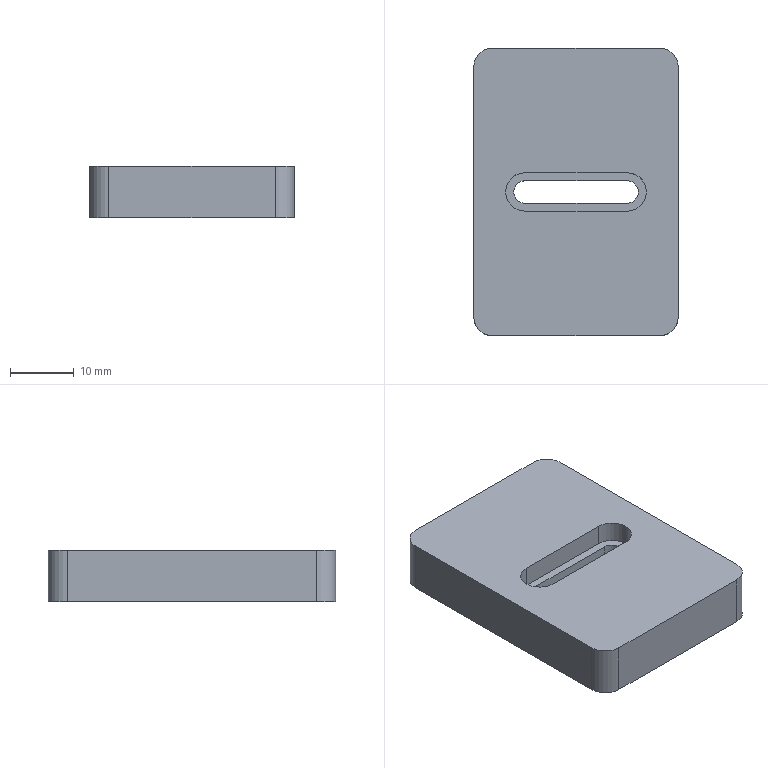Part | SolidWorks | features HoleWzd 2, ICE 2, Extrusion 1, Fillet 1 | 1 solid | 21 faces | box 32 x 45 x 8 mm | volume 10740 mm3 | plane 11 | cylinder 10 | commonest cylinder face diameters 6 x7 3.5 x3
STEP:
#1=CARTESIAN_POINT('',(11.,0.,4.7));
#2=VERTEX_POINT('',#1);
#3=CARTESIAN_POINT('',(8.,3.,4.7));
#4=VERTEX_POINT('',#3);
#5=CARTESIAN_POINT('',(8.,0.,4.7));
#6=DIRECTION('',(0.,0.,1.));
#7=DIRECTION('',(1.,0.,0.));
#8=AXIS2_PLACEMENT_3D('',#5,#6,#7);
#9=CIRCLE('',#8,3.);
#10=EDGE_CURVE('',#2,#4,#9,.T.);
#11=ORIENTED_EDGE('',*,*,#10,.F.);
#12=CARTESIAN_POINT('',(11.,0.,8.));
#13=VERTEX_POINT('',#12);
#14=CARTESIAN_POINT('',(11.,0.,4.7));
#15=DIRECTION('',(0.,0.,1.));
#16=VECTOR('',#15,1000.);
#17=LINE('',#14,#16);
#18=EDGE_CURVE('',#2,#13,#17,.T.);
#19=ORIENTED_EDGE('',*,*,#18,.T.);
#20=CARTESIAN_POINT('',(8.,3.,8.));
#21=VERTEX_POINT('',#20);
#22=CARTESIAN_POINT('',(8.,0.,8.));
#23=DIRECTION('',(0.,0.,1.));
#24=DIRECTION('',(1.,0.,0.));
#25=AXIS2_PLACEMENT_3D('',#22,#23,#24);
#26=CIRCLE('',#25,3.);
#27=EDGE_CURVE('',#13,#21,#26,.T.);
#28=ORIENTED_EDGE('',*,*,#27,.T.);
#29=CARTESIAN_POINT('',(8.,3.,4.7));
#30=DIRECTION('',(0.,0.,1.));
#31=VECTOR('',#30,1000.);
#32=LINE('',#29,#31);
#33=EDGE_CURVE('',#4,#21,#32,.T.);
#34=ORIENTED_EDGE('',*,*,#33,.F.);
#35=EDGE_LOOP('',(#11,#19,#28,#34));
#36=FACE_OUTER_BOUND('',#35,.T.);
#37=CARTESIAN_POINT('',(8.,0.,4.7));
#38=DIRECTION('',(0.,0.,1.));
#39=DIRECTION('',(1.,0.,0.));
#40=AXIS2_PLACEMENT_3D('',#37,#38,#39);
#41=CYLINDRICAL_SURFACE('',#40,3.);
#42=ADVANCED_FACE('',(#36),#41,.F.);
#43=CARTESIAN_POINT('',(9.75,0.,0.));
#44=VERTEX_POINT('',#43);
#45=CARTESIAN_POINT('',(8.,1.75,0.));
#46=VERTEX_POINT('',#45);
#47=CARTESIAN_POINT('',(8.,0.,0.));
#48=DIRECTION('',(0.,0.,1.));
#49=DIRECTION('',(1.,0.,0.));
#50=AXIS2_PLACEMENT_3D('',#47,#48,#49);
#51=CIRCLE('',#50,1.75);
#52=EDGE_CURVE('',#44,#46,#51,.T.);
#53=ORIENTED_EDGE('',*,*,#52,.F.);
#54=CARTESIAN_POINT('',(9.75,0.,4.7));
#55=VERTEX_POINT('',#54);
#56=CARTESIAN_POINT('',(9.75,0.,0.));
#57=DIRECTION('',(0.,0.,1.));
#58=VECTOR('',#57,1000.);
#59=LINE('',#56,#58);
#60=EDGE_CURVE('',#44,#55,#59,.T.);
#61=ORIENTED_EDGE('',*,*,#60,.T.);
#62=CARTESIAN_POINT('',(8.,1.75,4.7));
#63=VERTEX_POINT('',#62);
#64=CARTESIAN_POINT('',(8.,0.,4.7));
#65=DIRECTION('',(0.,0.,-1.));
#66=DIRECTION('',(1.,0.,0.));
#67=AXIS2_PLACEMENT_3D('',#64,#65,#66);
#68=CIRCLE('',#67,1.75);
#69=EDGE_CURVE('',#63,#55,#68,.T.);
#70=ORIENTED_EDGE('',*,*,#69,.F.);
#71=CARTESIAN_POINT('',(8.,1.75,0.));
#72=DIRECTION('',(0.,0.,1.));
#73=VECTOR('',#72,1000.);
#74=LINE('',#71,#73);
#75=EDGE_CURVE('',#46,#63,#74,.T.);
#76=ORIENTED_EDGE('',*,*,#75,.F.);
#77=EDGE_LOOP('',(#53,#61,#70,#76));
#78=FACE_OUTER_BOUND('',#77,.T.);
#79=CARTESIAN_POINT('',(8.,0.,0.));
#80=DIRECTION('',(0.,0.,1.));
#81=DIRECTION('',(1.,0.,0.));
#82=AXIS2_PLACEMENT_3D('',#79,#80,#81);
#83=CYLINDRICAL_SURFACE('',#82,1.75);
#84=ADVANCED_FACE('',(#78),#83,.F.);
#85=CARTESIAN_POINT('',(-8.,-1.75,4.7));
#86=VERTEX_POINT('',#85);
#87=CARTESIAN_POINT('',(-8.,1.75,4.7));
#88=VERTEX_POINT('',#87);
#89=CARTESIAN_POINT('',(-8.,0.,4.7));
#90=DIRECTION('',(0.,0.,-1.));
#91=DIRECTION('',(1.,0.,0.));
#92=AXIS2_PLACEMENT_3D('',#89,#90,#91);
#93=CIRCLE('',#92,1.75);
#94=EDGE_CURVE('',#86,#88,#93,.T.);
#95=ORIENTED_EDGE('',*,*,#94,.F.);
#96=CARTESIAN_POINT('',(-8.,-1.75,0.));
#97=VERTEX_POINT('',#96);
#98=CARTESIAN_POINT('',(-8.,-1.75,0.));
#99=DIRECTION('',(0.,0.,1.));
#100=VECTOR('',#99,1000.);
#101=LINE('',#98,#100);
#102=EDGE_CURVE('',#97,#86,#101,.T.);
#103=ORIENTED_EDGE('',*,*,#102,.F.);
#104=CARTESIAN_POINT('',(-8.,1.75,0.));
#105=VERTEX_POINT('',#104);
#106=CARTESIAN_POINT('',(-8.,0.,0.));
#107=DIRECTION('',(0.,0.,1.));
#108=DIRECTION('',(1.,0.,0.));
#109=AXIS2_PLACEMENT_3D('',#106,#107,#108);
#110=CIRCLE('',#109,1.75);
#111=EDGE_CURVE('',#105,#97,#110,.T.);
#112=ORIENTED_EDGE('',*,*,#111,.F.);
#113=CARTESIAN_POINT('',(-8.,1.75,0.));
#114=DIRECTION('',(0.,0.,1.));
#115=VECTOR('',#114,1000.);
#116=LINE('',#113,#115);
#117=EDGE_CURVE('',#105,#88,#116,.T.);
#118=ORIENTED_EDGE('',*,*,#117,.T.);
#119=EDGE_LOOP('',(#95,#103,#112,#118));
#120=FACE_OUTER_BOUND('',#119,.T.);
#121=CARTESIAN_POINT('',(-8.,0.,0.));
#122=DIRECTION('',(0.,0.,1.));
#123=DIRECTION('',(1.,0.,0.));
#124=AXIS2_PLACEMENT_3D('',#121,#122,#123);
#125=CYLINDRICAL_SURFACE('',#124,1.75);
#126=ADVANCED_FACE('',(#120),#125,.F.);
#127=CARTESIAN_POINT('',(-8.,1.75,4.7));
#128=DIRECTION('',(1.,0.,0.));
#129=VECTOR('',#128,1000.);
#130=LINE('',#127,#129);
#131=EDGE_CURVE('',#88,#63,#130,.T.);
#132=ORIENTED_EDGE('',*,*,#131,.F.);
#133=ORIENTED_EDGE('',*,*,#117,.F.);
#134=CARTESIAN_POINT('',(-8.,1.75,0.));
#135=DIRECTION('',(-1.,0.,0.));
#136=VECTOR('',#135,1000.);
#137=LINE('',#134,#136);
#138=EDGE_CURVE('',#46,#105,#137,.T.);
#139=ORIENTED_EDGE('',*,*,#138,.F.);
#140=ORIENTED_EDGE('',*,*,#75,.T.);
#141=EDGE_LOOP('',(#132,#133,#139,#140));
#142=FACE_OUTER_BOUND('',#141,.T.);
#143=CARTESIAN_POINT('',(-8.,1.75,0.));
#144=DIRECTION('',(0.,1.,0.));
#145=DIRECTION('',(0.,0.,1.));
#146=AXIS2_PLACEMENT_3D('',#143,#144,#145);
#147=PLANE('',#146);
#148=ADVANCED_FACE('',(#142),#147,.F.);
#149=ORIENTED_EDGE('',*,*,#60,.F.);
#150=CARTESIAN_POINT('',(8.,-1.75,0.));
#151=VERTEX_POINT('',#150);
#152=CARTESIAN_POINT('',(8.,0.,0.));
#153=DIRECTION('',(0.,0.,1.));
#154=DIRECTION('',(1.,0.,0.));
#155=AXIS2_PLACEMENT_3D('',#152,#153,#154);
#156=CIRCLE('',#155,1.75);
#157=EDGE_CURVE('',#151,#44,#156,.T.);
#158=ORIENTED_EDGE('',*,*,#157,.F.);
#159=CARTESIAN_POINT('',(8.,-1.75,4.7));
#160=VERTEX_POINT('',#159);
#161=CARTESIAN_POINT('',(8.,-1.75,0.));
#162=DIRECTION('',(0.,0.,1.));
#163=VECTOR('',#162,1000.);
#164=LINE('',#161,#163);
#165=EDGE_CURVE('',#151,#160,#164,.T.);
#166=ORIENTED_EDGE('',*,*,#165,.T.);
#167=CARTESIAN_POINT('',(8.,0.,4.7));
#168=DIRECTION('',(0.,0.,-1.));
#169=DIRECTION('',(1.,0.,0.));
#170=AXIS2_PLACEMENT_3D('',#167,#168,#169);
#171=CIRCLE('',#170,1.75);
#172=EDGE_CURVE('',#55,#160,#171,.T.);
#173=ORIENTED_EDGE('',*,*,#172,.F.);
#174=EDGE_LOOP('',(#149,#158,#166,#173));
#175=FACE_OUTER_BOUND('',#174,.T.);
#176=CARTESIAN_POINT('',(8.,0.,0.));
#177=DIRECTION('',(0.,0.,1.));
#178=DIRECTION('',(1.,0.,0.));
#179=AXIS2_PLACEMENT_3D('',#176,#177,#178);
#180=CYLINDRICAL_SURFACE('',#179,1.75);
#181=ADVANCED_FACE('',(#175),#180,.F.);
#182=CARTESIAN_POINT('',(-8.,-1.75,4.7));
#183=DIRECTION('',(-1.,0.,0.));
#184=VECTOR('',#183,1000.);
#185=LINE('',#182,#184);
#186=EDGE_CURVE('',#160,#86,#185,.T.);
#187=ORIENTED_EDGE('',*,*,#186,.F.);
#188=ORIENTED_EDGE('',*,*,#165,.F.);
#189=CARTESIAN_POINT('',(-8.,-1.75,0.));
#190=DIRECTION('',(1.,0.,0.));
#191=VECTOR('',#190,1000.);
#192=LINE('',#189,#191);
#193=EDGE_CURVE('',#97,#151,#192,.T.);
#194=ORIENTED_EDGE('',*,*,#193,.F.);
#195=ORIENTED_EDGE('',*,*,#102,.T.);
#196=EDGE_LOOP('',(#187,#188,#194,#195));
#197=FACE_OUTER_BOUND('',#196,.T.);
#198=CARTESIAN_POINT('',(-8.,-1.75,0.));
#199=DIRECTION('',(0.,-1.,0.));
#200=DIRECTION('',(0.,0.,-1.));
#201=AXIS2_PLACEMENT_3D('',#198,#199,#200);
#202=PLANE('',#201);
#203=ADVANCED_FACE('',(#197),#202,.F.);
#204=CARTESIAN_POINT('',(-16.,19.5,8.));
#205=VERTEX_POINT('',#204);
#206=CARTESIAN_POINT('',(-16.,-19.5,8.));
#207=VERTEX_POINT('',#206);
#208=CARTESIAN_POINT('',(-16.,-22.5,8.));
#209=DIRECTION('',(0.,-1.,0.));
#210=VECTOR('',#209,1000.);
#211=LINE('',#208,#210);
#212=EDGE_CURVE('',#205,#207,#211,.T.);
#213=ORIENTED_EDGE('',*,*,#212,.F.);
#214=CARTESIAN_POINT('',(-16.,19.5,0.));
#215=VERTEX_POINT('',#214);
#216=CARTESIAN_POINT('',(-16.,19.5,8.));
#217=DIRECTION('',(0.,0.,-1.));
#218=VECTOR('',#217,1000.);
#219=LINE('',#216,#218);
#220=EDGE_CURVE('',#205,#215,#219,.T.);
#221=ORIENTED_EDGE('',*,*,#220,.T.);
#222=CARTESIAN_POINT('',(-16.,-19.5,0.));
#223=VERTEX_POINT('',#222);
#224=CARTESIAN_POINT('',(-16.,-22.5,0.));
#225=DIRECTION('',(0.,-1.,0.));
#226=VECTOR('',#225,1000.);
#227=LINE('',#224,#226);
#228=EDGE_CURVE('',#215,#223,#227,.T.);
#229=ORIENTED_EDGE('',*,*,#228,.T.);
#230=CARTESIAN_POINT('',(-16.,-19.5,8.));
#231=DIRECTION('',(0.,0.,1.));
#232=VECTOR('',#231,1000.);
#233=LINE('',#230,#232);
#234=EDGE_CURVE('',#223,#207,#233,.T.);
#235=ORIENTED_EDGE('',*,*,#234,.T.);
#236=EDGE_LOOP('',(#213,#221,#229,#235));
#237=FACE_OUTER_BOUND('',#236,.T.);
#238=CARTESIAN_POINT('',(-16.,-22.5,8.));
#239=DIRECTION('',(1.,0.,0.));
#240=DIRECTION('',(0.,0.,-1.));
#241=AXIS2_PLACEMENT_3D('',#238,#239,#240);
#242=PLANE('',#241);
#243=ADVANCED_FACE('',(#237),#242,.F.);
#244=CARTESIAN_POINT('',(-13.,-22.5,0.));
#245=VERTEX_POINT('',#244);
#246=CARTESIAN_POINT('',(13.,-22.5,0.));
#247=VERTEX_POINT('',#246);
#248=CARTESIAN_POINT('',(16.,-22.5,0.));
#249=DIRECTION('',(1.,0.,0.));
#250=VECTOR('',#249,1000.);
#251=LINE('',#248,#250);
#252=EDGE_CURVE('',#245,#247,#251,.T.);
#253=ORIENTED_EDGE('',*,*,#252,.T.);
#254=CARTESIAN_POINT('',(13.,-22.5,8.));
#255=VERTEX_POINT('',#254);
#256=CARTESIAN_POINT('',(13.,-22.5,8.));
#257=DIRECTION('',(0.,0.,1.));
#258=VECTOR('',#257,1000.);
#259=LINE('',#256,#258);
#260=EDGE_CURVE('',#247,#255,#259,.T.);
#261=ORIENTED_EDGE('',*,*,#260,.T.);
#262=CARTESIAN_POINT('',(-13.,-22.5,8.));
#263=VERTEX_POINT('',#262);
#264=CARTESIAN_POINT('',(16.,-22.5,8.));
#265=DIRECTION('',(1.,0.,0.));
#266=VECTOR('',#265,1000.);
#267=LINE('',#264,#266);
#268=EDGE_CURVE('',#263,#255,#267,.T.);
#269=ORIENTED_EDGE('',*,*,#268,.F.);
#270=CARTESIAN_POINT('',(-13.,-22.5,8.));
#271=DIRECTION('',(0.,0.,-1.));
#272=VECTOR('',#271,1000.);
#273=LINE('',#270,#272);
#274=EDGE_CURVE('',#263,#245,#273,.T.);
#275=ORIENTED_EDGE('',*,*,#274,.T.);
#276=EDGE_LOOP('',(#253,#261,#269,#275));
#277=FACE_OUTER_BOUND('',#276,.T.);
#278=CARTESIAN_POINT('',(16.,-22.5,8.));
#279=DIRECTION('',(0.,1.,0.));
#280=DIRECTION('',(-1.,0.,0.));
#281=AXIS2_PLACEMENT_3D('',#278,#279,#280);
#282=PLANE('',#281);
#283=ADVANCED_FACE('',(#277),#282,.F.);
#284=CARTESIAN_POINT('',(16.,-19.5,0.));
#285=VERTEX_POINT('',#284);
#286=CARTESIAN_POINT('',(16.,19.5,0.));
#287=VERTEX_POINT('',#286);
#288=CARTESIAN_POINT('',(16.,-22.5,0.));
#289=DIRECTION('',(0.,1.,0.));
#290=VECTOR('',#289,1000.);
#291=LINE('',#288,#290);
#292=EDGE_CURVE('',#285,#287,#291,.T.);
#293=ORIENTED_EDGE('',*,*,#292,.T.);
#294=CARTESIAN_POINT('',(16.,19.5,8.));
#295=VERTEX_POINT('',#294);
#296=CARTESIAN_POINT('',(16.,19.5,8.));
#297=DIRECTION('',(0.,0.,1.));
#298=VECTOR('',#297,1000.);
#299=LINE('',#296,#298);
#300=EDGE_CURVE('',#287,#295,#299,.T.);
#301=ORIENTED_EDGE('',*,*,#300,.T.);
#302=CARTESIAN_POINT('',(16.,-19.5,8.));
#303=VERTEX_POINT('',#302);
#304=CARTESIAN_POINT('',(16.,-22.5,8.));
#305=DIRECTION('',(0.,1.,0.));
#306=VECTOR('',#305,1000.);
#307=LINE('',#304,#306);
#308=EDGE_CURVE('',#303,#295,#307,.T.);
#309=ORIENTED_EDGE('',*,*,#308,.F.);
#310=CARTESIAN_POINT('',(16.,-19.5,8.));
#311=DIRECTION('',(0.,0.,-1.));
#312=VECTOR('',#311,1000.);
#313=LINE('',#310,#312);
#314=EDGE_CURVE('',#303,#285,#313,.T.);
#315=ORIENTED_EDGE('',*,*,#314,.T.);
#316=EDGE_LOOP('',(#293,#301,#309,#315));
#317=FACE_OUTER_BOUND('',#316,.T.);
#318=CARTESIAN_POINT('',(16.,-22.5,8.));
#319=DIRECTION('',(-1.,0.,0.));
#320=DIRECTION('',(0.,0.,1.));
#321=AXIS2_PLACEMENT_3D('',#318,#319,#320);
#322=PLANE('',#321);
#323=ADVANCED_FACE('',(#317),#322,.F.);
#324=CARTESIAN_POINT('',(13.,22.5,0.));
#325=VERTEX_POINT('',#324);
#326=CARTESIAN_POINT('',(-13.,22.5,0.));
#327=VERTEX_POINT('',#326);
#328=CARTESIAN_POINT('',(16.,22.5,0.));
#329=DIRECTION('',(-1.,0.,0.));
#330=VECTOR('',#329,1000.);
#331=LINE('',#328,#330);
#332=EDGE_CURVE('',#325,#327,#331,.T.);
#333=ORIENTED_EDGE('',*,*,#332,.T.);
#334=CARTESIAN_POINT('',(-13.,22.5,8.));
#335=VERTEX_POINT('',#334);
#336=CARTESIAN_POINT('',(-13.,22.5,8.));
#337=DIRECTION('',(0.,0.,1.));
#338=VECTOR('',#337,1000.);
#339=LINE('',#336,#338);
#340=EDGE_CURVE('',#327,#335,#339,.T.);
#341=ORIENTED_EDGE('',*,*,#340,.T.);
#342=CARTESIAN_POINT('',(13.,22.5,8.));
#343=VERTEX_POINT('',#342);
#344=CARTESIAN_POINT('',(16.,22.5,8.));
#345=DIRECTION('',(-1.,0.,0.));
#346=VECTOR('',#345,1000.);
#347=LINE('',#344,#346);
#348=EDGE_CURVE('',#343,#335,#347,.T.);
#349=ORIENTED_EDGE('',*,*,#348,.F.);
#350=CARTESIAN_POINT('',(13.,22.5,8.));
#351=DIRECTION('',(0.,0.,-1.));
#352=VECTOR('',#351,1000.);
#353=LINE('',#350,#352);
#354=EDGE_CURVE('',#343,#325,#353,.T.);
#355=ORIENTED_EDGE('',*,*,#354,.T.);
#356=EDGE_LOOP('',(#333,#341,#349,#355));
#357=FACE_OUTER_BOUND('',#356,.T.);
#358=CARTESIAN_POINT('',(16.,22.5,8.));
#359=DIRECTION('',(0.,-1.,0.));
#360=DIRECTION('',(1.,0.,0.));
#361=AXIS2_PLACEMENT_3D('',#358,#359,#360);
#362=PLANE('',#361);
#363=ADVANCED_FACE('',(#357),#362,.F.);
#364=CARTESIAN_POINT('',(-8.,3.,8.));
#365=VERTEX_POINT('',#364);
#366=CARTESIAN_POINT('',(-8.,-3.,8.));
#367=VERTEX_POINT('',#366);
#368=CARTESIAN_POINT('',(-8.,0.,8.));
#369=DIRECTION('',(0.,0.,1.));
#370=DIRECTION('',(1.,0.,0.));
#371=AXIS2_PLACEMENT_3D('',#368,#369,#370);
#372=CIRCLE('',#371,3.);
#373=EDGE_CURVE('',#365,#367,#372,.T.);
#374=ORIENTED_EDGE('',*,*,#373,.F.);
#375=CARTESIAN_POINT('',(-8.,3.,8.));
#376=DIRECTION('',(-1.,0.,0.));
#377=VECTOR('',#376,1000.);
#378=LINE('',#375,#377);
#379=EDGE_CURVE('',#21,#365,#378,.T.);
#380=ORIENTED_EDGE('',*,*,#379,.F.);
#381=ORIENTED_EDGE('',*,*,#27,.F.);
#382=CARTESIAN_POINT('',(8.,-3.,8.));
#383=VERTEX_POINT('',#382);
#384=CARTESIAN_POINT('',(8.,0.,8.));
#385=DIRECTION('',(0.,0.,1.));
#386=DIRECTION('',(1.,0.,0.));
#387=AXIS2_PLACEMENT_3D('',#384,#385,#386);
#388=CIRCLE('',#387,3.);
#389=EDGE_CURVE('',#383,#13,#388,.T.);
#390=ORIENTED_EDGE('',*,*,#389,.F.);
#391=CARTESIAN_POINT('',(-8.,-3.,8.));
#392=DIRECTION('',(1.,0.,0.));
#393=VECTOR('',#392,1000.);
#394=LINE('',#391,#393);
#395=EDGE_CURVE('',#367,#383,#394,.T.);
#396=ORIENTED_EDGE('',*,*,#395,.F.);
#397=EDGE_LOOP('',(#374,#380,#381,#390,#396));
#398=FACE_BOUND('',#397,.T.);
#399=ORIENTED_EDGE('',*,*,#348,.T.);
#400=CARTESIAN_POINT('',(-13.,19.5,8.));
#401=DIRECTION('',(0.,0.,1.));
#402=DIRECTION('',(1.,0.,0.));
#403=AXIS2_PLACEMENT_3D('',#400,#401,#402);
#404=CIRCLE('',#403,3.);
#405=EDGE_CURVE('',#335,#205,#404,.T.);
#406=ORIENTED_EDGE('',*,*,#405,.T.);
#407=ORIENTED_EDGE('',*,*,#212,.T.);
#408=CARTESIAN_POINT('',(-13.,-19.5,8.));
#409=DIRECTION('',(0.,0.,1.));
#410=DIRECTION('',(1.,0.,0.));
#411=AXIS2_PLACEMENT_3D('',#408,#409,#410);
#412=CIRCLE('',#411,3.);
#413=EDGE_CURVE('',#207,#263,#412,.T.);
#414=ORIENTED_EDGE('',*,*,#413,.T.);
#415=ORIENTED_EDGE('',*,*,#268,.T.);
#416=CARTESIAN_POINT('',(13.,-19.5,8.));
#417=DIRECTION('',(0.,0.,1.));
#418=DIRECTION('',(1.,0.,0.));
#419=AXIS2_PLACEMENT_3D('',#416,#417,#418);
#420=CIRCLE('',#419,3.);
#421=EDGE_CURVE('',#255,#303,#420,.T.);
#422=ORIENTED_EDGE('',*,*,#421,.T.);
#423=ORIENTED_EDGE('',*,*,#308,.T.);
#424=CARTESIAN_POINT('',(13.,19.5,8.));
#425=DIRECTION('',(0.,0.,1.));
#426=DIRECTION('',(1.,0.,0.));
#427=AXIS2_PLACEMENT_3D('',#424,#425,#426);
#428=CIRCLE('',#427,3.);
#429=EDGE_CURVE('',#295,#343,#428,.T.);
#430=ORIENTED_EDGE('',*,*,#429,.T.);
#431=EDGE_LOOP('',(#399,#406,#407,#414,#415,#422,#423,#430));
#432=FACE_OUTER_BOUND('',#431,.T.);
#433=CARTESIAN_POINT('',(0.,0.,8.));
#434=DIRECTION('',(0.,0.,1.));
#435=DIRECTION('',(1.,0.,0.));
#436=AXIS2_PLACEMENT_3D('',#433,#434,#435);
#437=PLANE('',#436);
#438=ADVANCED_FACE('',(#398,#432),#437,.T.);
#439=ORIENTED_EDGE('',*,*,#138,.T.);
#440=ORIENTED_EDGE('',*,*,#111,.T.);
#441=ORIENTED_EDGE('',*,*,#193,.T.);
#442=ORIENTED_EDGE('',*,*,#157,.T.);
#443=ORIENTED_EDGE('',*,*,#52,.T.);
#444=EDGE_LOOP('',(#439,#440,#441,#442,#443));
#445=FACE_BOUND('',#444,.T.);
#446=ORIENTED_EDGE('',*,*,#228,.F.);
#447=CARTESIAN_POINT('',(-13.,19.5,0.));
#448=DIRECTION('',(0.,0.,-1.));
#449=DIRECTION('',(1.,0.,0.));
#450=AXIS2_PLACEMENT_3D('',#447,#448,#449);
#451=CIRCLE('',#450,3.);
#452=EDGE_CURVE('',#215,#327,#451,.T.);
#453=ORIENTED_EDGE('',*,*,#452,.T.);
#454=ORIENTED_EDGE('',*,*,#332,.F.);
#455=CARTESIAN_POINT('',(13.,19.5,0.));
#456=DIRECTION('',(0.,0.,-1.));
#457=DIRECTION('',(1.,0.,0.));
#458=AXIS2_PLACEMENT_3D('',#455,#456,#457);
#459=CIRCLE('',#458,3.);
#460=EDGE_CURVE('',#325,#287,#459,.T.);
#461=ORIENTED_EDGE('',*,*,#460,.T.);
#462=ORIENTED_EDGE('',*,*,#292,.F.);
#463=CARTESIAN_POINT('',(13.,-19.5,0.));
#464=DIRECTION('',(0.,0.,-1.));
#465=DIRECTION('',(1.,0.,0.));
#466=AXIS2_PLACEMENT_3D('',#463,#464,#465);
#467=CIRCLE('',#466,3.);
#468=EDGE_CURVE('',#285,#247,#467,.T.);
#469=ORIENTED_EDGE('',*,*,#468,.T.);
#470=ORIENTED_EDGE('',*,*,#252,.F.);
#471=CARTESIAN_POINT('',(-13.,-19.5,0.));
#472=DIRECTION('',(0.,0.,-1.));
#473=DIRECTION('',(1.,0.,0.));
#474=AXIS2_PLACEMENT_3D('',#471,#472,#473);
#475=CIRCLE('',#474,3.);
#476=EDGE_CURVE('',#245,#223,#475,.T.);
#477=ORIENTED_EDGE('',*,*,#476,.T.);
#478=EDGE_LOOP('',(#446,#453,#454,#461,#462,#469,#470,#477));
#479=FACE_OUTER_BOUND('',#478,.T.);
#480=CARTESIAN_POINT('',(0.,0.,0.));
#481=DIRECTION('',(0.,0.,1.));
#482=DIRECTION('',(1.,0.,0.));
#483=AXIS2_PLACEMENT_3D('',#480,#481,#482);
#484=PLANE('',#483);
#485=ADVANCED_FACE('',(#445,#479),#484,.F.);
#486=CARTESIAN_POINT('',(-8.,3.,4.7));
#487=VERTEX_POINT('',#486);
#488=CARTESIAN_POINT('',(-8.,-3.,4.7));
#489=VERTEX_POINT('',#488);
#490=CARTESIAN_POINT('',(-8.,0.,4.7));
#491=DIRECTION('',(0.,0.,1.));
#492=DIRECTION('',(1.,0.,0.));
#493=AXIS2_PLACEMENT_3D('',#490,#491,#492);
#494=CIRCLE('',#493,3.);
#495=EDGE_CURVE('',#487,#489,#494,.T.);
#496=ORIENTED_EDGE('',*,*,#495,.T.);
#497=CARTESIAN_POINT('',(8.,-3.,4.7));
#498=VERTEX_POINT('',#497);
#499=CARTESIAN_POINT('',(-8.,-3.,4.7));
#500=DIRECTION('',(1.,0.,0.));
#501=VECTOR('',#500,1000.);
#502=LINE('',#499,#501);
#503=EDGE_CURVE('',#489,#498,#502,.T.);
#504=ORIENTED_EDGE('',*,*,#503,.T.);
#505=CARTESIAN_POINT('',(8.,0.,4.7));
#506=DIRECTION('',(0.,0.,1.));
#507=DIRECTION('',(1.,0.,0.));
#508=AXIS2_PLACEMENT_3D('',#505,#506,#507);
#509=CIRCLE('',#508,3.);
#510=EDGE_CURVE('',#498,#2,#509,.T.);
#511=ORIENTED_EDGE('',*,*,#510,.T.);
#512=ORIENTED_EDGE('',*,*,#10,.T.);
#513=CARTESIAN_POINT('',(-8.,3.,4.7));
#514=DIRECTION('',(-1.,0.,0.));
#515=VECTOR('',#514,1000.);
#516=LINE('',#513,#515);
#517=EDGE_CURVE('',#4,#487,#516,.T.);
#518=ORIENTED_EDGE('',*,*,#517,.T.);
#519=EDGE_LOOP('',(#496,#504,#511,#512,#518));
#520=FACE_OUTER_BOUND('',#519,.T.);
#521=ORIENTED_EDGE('',*,*,#94,.T.);
#522=ORIENTED_EDGE('',*,*,#131,.T.);
#523=ORIENTED_EDGE('',*,*,#69,.T.);
#524=ORIENTED_EDGE('',*,*,#172,.T.);
#525=ORIENTED_EDGE('',*,*,#186,.T.);
#526=EDGE_LOOP('',(#521,#522,#523,#524,#525));
#527=FACE_BOUND('',#526,.T.);
#528=CARTESIAN_POINT('',(-8.,0.,4.7));
#529=DIRECTION('',(0.,0.,1.));
#530=DIRECTION('',(1.,0.,0.));
#531=AXIS2_PLACEMENT_3D('',#528,#529,#530);
#532=PLANE('',#531);
#533=ADVANCED_FACE('',(#520,#527),#532,.T.);
#534=ORIENTED_EDGE('',*,*,#373,.T.);
#535=CARTESIAN_POINT('',(-8.,-3.,4.7));
#536=DIRECTION('',(0.,0.,1.));
#537=VECTOR('',#536,1000.);
#538=LINE('',#535,#537);
#539=EDGE_CURVE('',#489,#367,#538,.T.);
#540=ORIENTED_EDGE('',*,*,#539,.F.);
#541=ORIENTED_EDGE('',*,*,#495,.F.);
#542=CARTESIAN_POINT('',(-8.,3.,4.7));
#543=DIRECTION('',(0.,0.,1.));
#544=VECTOR('',#543,1000.);
#545=LINE('',#542,#544);
#546=EDGE_CURVE('',#487,#365,#545,.T.);
#547=ORIENTED_EDGE('',*,*,#546,.T.);
#548=EDGE_LOOP('',(#534,#540,#541,#547));
#549=FACE_OUTER_BOUND('',#548,.T.);
#550=CARTESIAN_POINT('',(-8.,0.,4.7));
#551=DIRECTION('',(0.,0.,1.));
#552=DIRECTION('',(1.,0.,0.));
#553=AXIS2_PLACEMENT_3D('',#550,#551,#552);
#554=CYLINDRICAL_SURFACE('',#553,3.);
#555=ADVANCED_FACE('',(#549),#554,.F.);
#556=ORIENTED_EDGE('',*,*,#379,.T.);
#557=ORIENTED_EDGE('',*,*,#546,.F.);
#558=ORIENTED_EDGE('',*,*,#517,.F.);
#559=ORIENTED_EDGE('',*,*,#33,.T.);
#560=EDGE_LOOP('',(#556,#557,#558,#559));
#561=FACE_OUTER_BOUND('',#560,.T.);
#562=CARTESIAN_POINT('',(-8.,3.,4.7));
#563=DIRECTION('',(0.,1.,0.));
#564=DIRECTION('',(0.,0.,1.));
#565=AXIS2_PLACEMENT_3D('',#562,#563,#564);
#566=PLANE('',#565);
#567=ADVANCED_FACE('',(#561),#566,.F.);
#568=ORIENTED_EDGE('',*,*,#18,.F.);
#569=ORIENTED_EDGE('',*,*,#510,.F.);
#570=CARTESIAN_POINT('',(8.,-3.,4.7));
#571=DIRECTION('',(0.,0.,1.));
#572=VECTOR('',#571,1000.);
#573=LINE('',#570,#572);
#574=EDGE_CURVE('',#498,#383,#573,.T.);
#575=ORIENTED_EDGE('',*,*,#574,.T.);
#576=ORIENTED_EDGE('',*,*,#389,.T.);
#577=EDGE_LOOP('',(#568,#569,#575,#576));
#578=FACE_OUTER_BOUND('',#577,.T.);
#579=CARTESIAN_POINT('',(8.,0.,4.7));
#580=DIRECTION('',(0.,0.,1.));
#581=DIRECTION('',(1.,0.,0.));
#582=AXIS2_PLACEMENT_3D('',#579,#580,#581);
#583=CYLINDRICAL_SURFACE('',#582,3.);
#584=ADVANCED_FACE('',(#578),#583,.F.);
#585=ORIENTED_EDGE('',*,*,#395,.T.);
#586=ORIENTED_EDGE('',*,*,#574,.F.);
#587=ORIENTED_EDGE('',*,*,#503,.F.);
#588=ORIENTED_EDGE('',*,*,#539,.T.);
#589=EDGE_LOOP('',(#585,#586,#587,#588));
#590=FACE_OUTER_BOUND('',#589,.T.);
#591=CARTESIAN_POINT('',(-8.,-3.,4.7));
#592=DIRECTION('',(0.,-1.,0.));
#593=DIRECTION('',(0.,0.,-1.));
#594=AXIS2_PLACEMENT_3D('',#591,#592,#593);
#595=PLANE('',#594);
#596=ADVANCED_FACE('',(#590),#595,.F.);
#597=ORIENTED_EDGE('',*,*,#405,.F.);
#598=ORIENTED_EDGE('',*,*,#340,.F.);
#599=ORIENTED_EDGE('',*,*,#452,.F.);
#600=ORIENTED_EDGE('',*,*,#220,.F.);
#601=EDGE_LOOP('',(#597,#598,#599,#600));
#602=FACE_OUTER_BOUND('',#601,.T.);
#603=CARTESIAN_POINT('',(-13.,19.5,8.));
#604=DIRECTION('',(0.,0.,-1.));
#605=DIRECTION('',(-1.,0.,0.));
#606=AXIS2_PLACEMENT_3D('',#603,#604,#605);
#607=CYLINDRICAL_SURFACE('',#606,3.);
#608=ADVANCED_FACE('',(#602),#607,.T.);
#609=ORIENTED_EDGE('',*,*,#429,.F.);
#610=ORIENTED_EDGE('',*,*,#300,.F.);
#611=ORIENTED_EDGE('',*,*,#460,.F.);
#612=ORIENTED_EDGE('',*,*,#354,.F.);
#613=EDGE_LOOP('',(#609,#610,#611,#612));
#614=FACE_OUTER_BOUND('',#613,.T.);
#615=CARTESIAN_POINT('',(13.,19.5,8.));
#616=DIRECTION('',(0.,0.,-1.));
#617=DIRECTION('',(-1.,0.,0.));
#618=AXIS2_PLACEMENT_3D('',#615,#616,#617);
#619=CYLINDRICAL_SURFACE('',#618,3.);
#620=ADVANCED_FACE('',(#614),#619,.T.);
#621=ORIENTED_EDGE('',*,*,#421,.F.);
#622=ORIENTED_EDGE('',*,*,#260,.F.);
#623=ORIENTED_EDGE('',*,*,#468,.F.);
#624=ORIENTED_EDGE('',*,*,#314,.F.);
#625=EDGE_LOOP('',(#621,#622,#623,#624));
#626=FACE_OUTER_BOUND('',#625,.T.);
#627=CARTESIAN_POINT('',(13.,-19.5,8.));
#628=DIRECTION('',(0.,0.,-1.));
#629=DIRECTION('',(-1.,0.,0.));
#630=AXIS2_PLACEMENT_3D('',#627,#628,#629);
#631=CYLINDRICAL_SURFACE('',#630,3.);
#632=ADVANCED_FACE('',(#626),#631,.T.);
#633=ORIENTED_EDGE('',*,*,#413,.F.);
#634=ORIENTED_EDGE('',*,*,#234,.F.);
#635=ORIENTED_EDGE('',*,*,#476,.F.);
#636=ORIENTED_EDGE('',*,*,#274,.F.);
#637=EDGE_LOOP('',(#633,#634,#635,#636));
#638=FACE_OUTER_BOUND('',#637,.T.);
#639=CARTESIAN_POINT('',(-13.,-19.5,8.));
#640=DIRECTION('',(0.,0.,-1.));
#641=DIRECTION('',(-1.,0.,0.));
#642=AXIS2_PLACEMENT_3D('',#639,#640,#641);
#643=CYLINDRICAL_SURFACE('',#642,3.);
#644=ADVANCED_FACE('',(#638),#643,.T.);
#645=CLOSED_SHELL('',(#42,#84,#126,#148,#181,#203,#243,#283,#323,#363,#438,#485,#533,#555,#567,#584,#596,#608,#620,#632,#644));
#646=MANIFOLD_SOLID_BREP('',#645);
#647=CARTESIAN_POINT('',(0.,0.,0.));
#648=DIRECTION('',(0.,0.,1.));
#649=DIRECTION('',(1.,0.,0.));
#650=AXIS2_PLACEMENT_3D('',#647,#648,#649);
#651=(LENGTH_UNIT()NAMED_UNIT(*)SI_UNIT(.MILLI.,.METRE.));
#652=UNCERTAINTY_MEASURE_WITH_UNIT(LENGTH_MEASURE(0.00001),#651,'','');
#653=(NAMED_UNIT(*)PLANE_ANGLE_UNIT()SI_UNIT($,.RADIAN.));
#654=(NAMED_UNIT(*)SI_UNIT($,.STERADIAN.)SOLID_ANGLE_UNIT());
#655=(GEOMETRIC_REPRESENTATION_CONTEXT(3)GLOBAL_UNCERTAINTY_ASSIGNED_CONTEXT((#652))GLOBAL_UNIT_ASSIGNED_CONTEXT((#651,#653,#654))REPRESENTATION_CONTEXT('',''));
#656=ADVANCED_BREP_SHAPE_REPRESENTATION('',(#646,#650),#655);